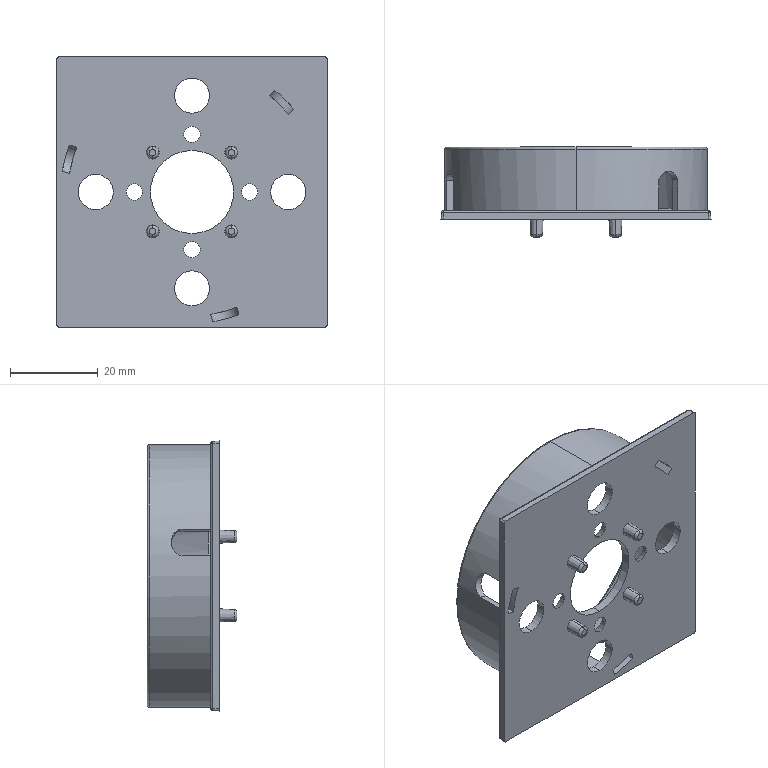Part | STEP file | PCS-P01B-2_1_2.stp | 1 solid | 88 faces | box 61.7 x 20.5 x 61.7 mm | volume 10976 mm3 | cylinder 29 | cone 20 | plane 19 | torus 12 | spline 8 | commonest cylinder face diameters 8 x8 56.5 x5 60 x5 1 x4 6.805 x3 19 x2